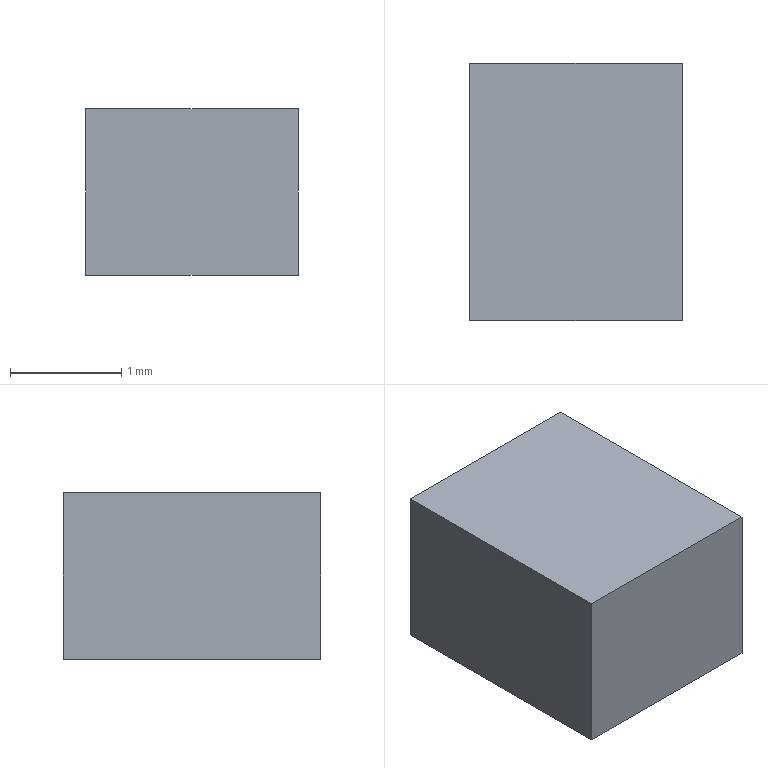Part | Creo | 1 solid | 6 faces | box 1.91 x 2.31 x 1.499 mm | volume 6.612 mm3 | plane 6
STEP:
#1=CARTESIAN_POINT('',(0.,0.,0.));
#2=DIRECTION('',(0.,0.,1.));
#3=DIRECTION('',(1.,0.,0.));
#4=AXIS2_PLACEMENT_3D('',#1,#2,#3);
#5=CARTESIAN_POINT('',(-0.955,-1.155,0.));
#6=VERTEX_POINT('',#5);
#7=CARTESIAN_POINT('',(0.955,-1.155,0.));
#8=VERTEX_POINT('',#7);
#9=CARTESIAN_POINT('',(-0.955,-1.155,0.));
#10=DIRECTION('',(1.,0.,0.));
#11=VECTOR('',#10,1.91);
#12=LINE('',#9,#11);
#13=EDGE_CURVE('',#6,#8,#12,.T.);
#14=ORIENTED_EDGE('',*,*,#13,.T.);
#15=CARTESIAN_POINT('',(0.955,1.155,0.));
#16=VERTEX_POINT('',#15);
#17=CARTESIAN_POINT('',(0.955,-1.155,0.));
#18=DIRECTION('',(0.,1.,0.));
#19=VECTOR('',#18,2.31);
#20=LINE('',#17,#19);
#21=EDGE_CURVE('',#8,#16,#20,.T.);
#22=ORIENTED_EDGE('',*,*,#21,.T.);
#23=CARTESIAN_POINT('',(-0.955,1.155,0.));
#24=VERTEX_POINT('',#23);
#25=CARTESIAN_POINT('',(0.955,1.155,0.));
#26=DIRECTION('',(-1.,0.,0.));
#27=VECTOR('',#26,1.91);
#28=LINE('',#25,#27);
#29=EDGE_CURVE('',#16,#24,#28,.T.);
#30=ORIENTED_EDGE('',*,*,#29,.T.);
#31=CARTESIAN_POINT('',(-0.955,1.155,0.));
#32=DIRECTION('',(0.,-1.,0.));
#33=VECTOR('',#32,2.31);
#34=LINE('',#31,#33);
#35=EDGE_CURVE('',#24,#6,#34,.T.);
#36=ORIENTED_EDGE('',*,*,#35,.T.);
#37=EDGE_LOOP('',(#14,#22,#30,#36));
#38=FACE_OUTER_BOUND('',#37,.F.);
#39=CARTESIAN_POINT('',(0.,0.,0.));
#40=DIRECTION('',(0.,0.,1.));
#41=DIRECTION('',(1.,0.,0.));
#42=AXIS2_PLACEMENT_3D('',#39,#40,#41);
#43=PLANE('',#42);
#44=ADVANCED_FACE('',(#38),#43,.F.);
#45=ORIENTED_EDGE('',*,*,#13,.F.);
#46=CARTESIAN_POINT('',(-0.955,-1.155,1.499));
#47=VERTEX_POINT('',#46);
#48=CARTESIAN_POINT('',(-0.955,-1.155,0.));
#49=DIRECTION('',(0.,0.,1.));
#50=VECTOR('',#49,1.499);
#51=LINE('',#48,#50);
#52=EDGE_CURVE('',#6,#47,#51,.T.);
#53=ORIENTED_EDGE('',*,*,#52,.T.);
#54=CARTESIAN_POINT('',(0.955,-1.155,1.499));
#55=VERTEX_POINT('',#54);
#56=CARTESIAN_POINT('',(-0.955,-1.155,1.499));
#57=DIRECTION('',(1.,0.,0.));
#58=VECTOR('',#57,1.91);
#59=LINE('',#56,#58);
#60=EDGE_CURVE('',#47,#55,#59,.T.);
#61=ORIENTED_EDGE('',*,*,#60,.T.);
#62=CARTESIAN_POINT('',(0.955,-1.155,0.));
#63=DIRECTION('',(0.,0.,1.));
#64=VECTOR('',#63,1.499);
#65=LINE('',#62,#64);
#66=EDGE_CURVE('',#8,#55,#65,.T.);
#67=ORIENTED_EDGE('',*,*,#66,.F.);
#68=EDGE_LOOP('',(#45,#53,#61,#67));
#69=FACE_OUTER_BOUND('',#68,.F.);
#70=CARTESIAN_POINT('',(-0.955,-1.155,0.));
#71=DIRECTION('',(0.,-1.,0.));
#72=DIRECTION('',(1.,0.,0.));
#73=AXIS2_PLACEMENT_3D('',#70,#71,#72);
#74=PLANE('',#73);
#75=ADVANCED_FACE('',(#69),#74,.T.);
#76=ORIENTED_EDGE('',*,*,#35,.F.);
#77=CARTESIAN_POINT('',(-0.955,1.155,1.499));
#78=VERTEX_POINT('',#77);
#79=CARTESIAN_POINT('',(-0.955,1.155,0.));
#80=DIRECTION('',(0.,0.,1.));
#81=VECTOR('',#80,1.499);
#82=LINE('',#79,#81);
#83=EDGE_CURVE('',#24,#78,#82,.T.);
#84=ORIENTED_EDGE('',*,*,#83,.T.);
#85=CARTESIAN_POINT('',(-0.955,1.155,1.499));
#86=DIRECTION('',(0.,-1.,0.));
#87=VECTOR('',#86,2.31);
#88=LINE('',#85,#87);
#89=EDGE_CURVE('',#78,#47,#88,.T.);
#90=ORIENTED_EDGE('',*,*,#89,.T.);
#91=ORIENTED_EDGE('',*,*,#52,.F.);
#92=EDGE_LOOP('',(#76,#84,#90,#91));
#93=FACE_OUTER_BOUND('',#92,.F.);
#94=CARTESIAN_POINT('',(-0.955,1.155,0.));
#95=DIRECTION('',(-1.,0.,0.));
#96=DIRECTION('',(0.,-1.,0.));
#97=AXIS2_PLACEMENT_3D('',#94,#95,#96);
#98=PLANE('',#97);
#99=ADVANCED_FACE('',(#93),#98,.T.);
#100=ORIENTED_EDGE('',*,*,#29,.F.);
#101=CARTESIAN_POINT('',(0.955,1.155,1.499));
#102=VERTEX_POINT('',#101);
#103=CARTESIAN_POINT('',(0.955,1.155,0.));
#104=DIRECTION('',(0.,0.,1.));
#105=VECTOR('',#104,1.499);
#106=LINE('',#103,#105);
#107=EDGE_CURVE('',#16,#102,#106,.T.);
#108=ORIENTED_EDGE('',*,*,#107,.T.);
#109=CARTESIAN_POINT('',(0.955,1.155,1.499));
#110=DIRECTION('',(-1.,0.,0.));
#111=VECTOR('',#110,1.91);
#112=LINE('',#109,#111);
#113=EDGE_CURVE('',#102,#78,#112,.T.);
#114=ORIENTED_EDGE('',*,*,#113,.T.);
#115=ORIENTED_EDGE('',*,*,#83,.F.);
#116=EDGE_LOOP('',(#100,#108,#114,#115));
#117=FACE_OUTER_BOUND('',#116,.F.);
#118=CARTESIAN_POINT('',(0.955,1.155,0.));
#119=DIRECTION('',(0.,1.,0.));
#120=DIRECTION('',(-1.,0.,0.));
#121=AXIS2_PLACEMENT_3D('',#118,#119,#120);
#122=PLANE('',#121);
#123=ADVANCED_FACE('',(#117),#122,.T.);
#124=ORIENTED_EDGE('',*,*,#21,.F.);
#125=ORIENTED_EDGE('',*,*,#66,.T.);
#126=CARTESIAN_POINT('',(0.955,-1.155,1.499));
#127=DIRECTION('',(0.,1.,0.));
#128=VECTOR('',#127,2.31);
#129=LINE('',#126,#128);
#130=EDGE_CURVE('',#55,#102,#129,.T.);
#131=ORIENTED_EDGE('',*,*,#130,.T.);
#132=ORIENTED_EDGE('',*,*,#107,.F.);
#133=EDGE_LOOP('',(#124,#125,#131,#132));
#134=FACE_OUTER_BOUND('',#133,.F.);
#135=CARTESIAN_POINT('',(0.955,-1.155,0.));
#136=DIRECTION('',(1.,0.,0.));
#137=DIRECTION('',(0.,1.,0.));
#138=AXIS2_PLACEMENT_3D('',#135,#136,#137);
#139=PLANE('',#138);
#140=ADVANCED_FACE('',(#134),#139,.T.);
#141=ORIENTED_EDGE('',*,*,#60,.F.);
#142=ORIENTED_EDGE('',*,*,#89,.F.);
#143=ORIENTED_EDGE('',*,*,#113,.F.);
#144=ORIENTED_EDGE('',*,*,#130,.F.);
#145=EDGE_LOOP('',(#141,#142,#143,#144));
#146=FACE_OUTER_BOUND('',#145,.F.);
#147=CARTESIAN_POINT('',(0.,0.,1.499));
#148=DIRECTION('',(0.,0.,1.));
#149=DIRECTION('',(1.,0.,0.));
#150=AXIS2_PLACEMENT_3D('',#147,#148,#149);
#151=PLANE('',#150);
#152=ADVANCED_FACE('',(#146),#151,.T.);
#153=CLOSED_SHELL('',(#44,#75,#99,#123,#140,#152));
#154=MANIFOLD_SOLID_BREP('',#153);
#155=(LENGTH_UNIT()NAMED_UNIT(*)SI_UNIT(.MILLI.,.METRE.));
#156=UNCERTAINTY_MEASURE_WITH_UNIT(LENGTH_MEASURE(0.0003351),#155,'','');
#157=(NAMED_UNIT(*)PLANE_ANGLE_UNIT()SI_UNIT($,.RADIAN.));
#158=PLANE_ANGLE_MEASURE_WITH_UNIT(PLANE_ANGLE_MEASURE(0.01745),#157);
#159=(CONVERSION_BASED_UNIT('DEGREE',#158)NAMED_UNIT(*)PLANE_ANGLE_UNIT());
#160=(NAMED_UNIT(*)SI_UNIT($,.STERADIAN.)SOLID_ANGLE_UNIT());
#161=(GEOMETRIC_REPRESENTATION_CONTEXT(3)GLOBAL_UNCERTAINTY_ASSIGNED_CONTEXT((#156))GLOBAL_UNIT_ASSIGNED_CONTEXT((#155,#159,#160))REPRESENTATION_CONTEXT('',''));
#162=ADVANCED_BREP_SHAPE_REPRESENTATION('',(#4,#154),#161);